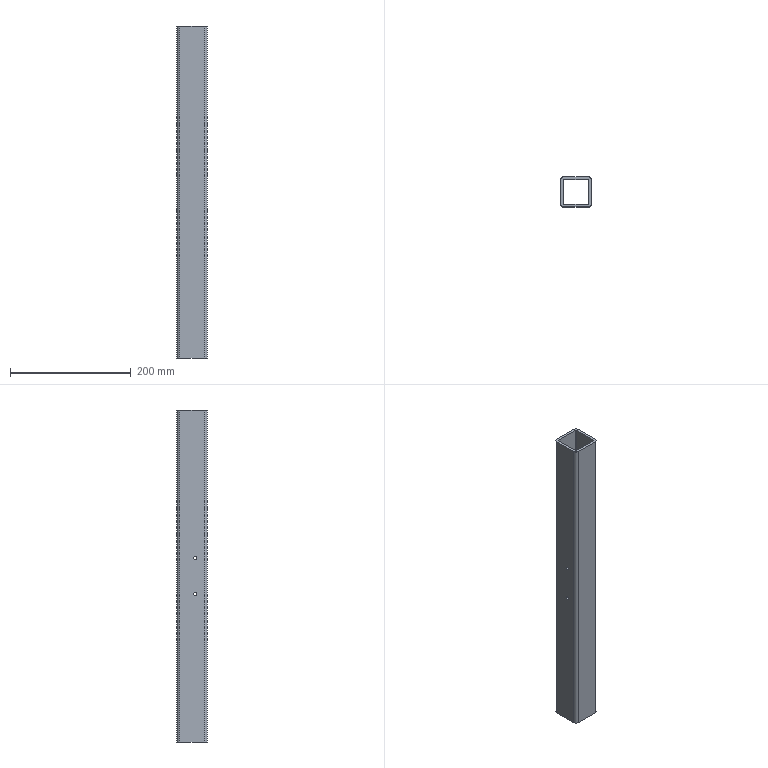Part | STEP file | Square steel 50×50×550 | 1 solid | 26 faces | box 50 x 50 x 550 mm | volume 393155 mm3 | cylinder 16 | plane 10 | commonest cylinder face diameters 5 x8 2 x4 10 x4